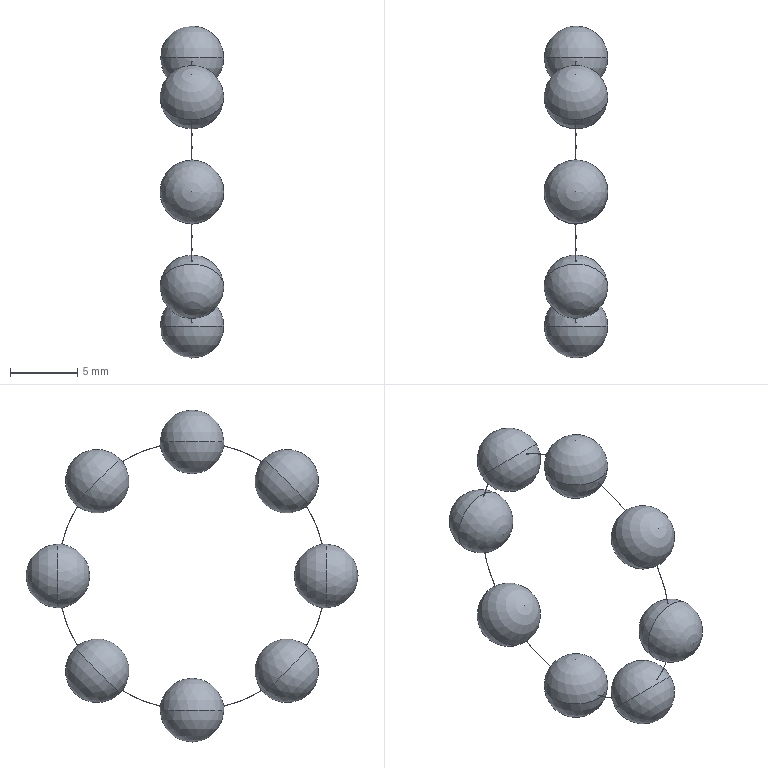Part | SolidWorks | features BaseBody 1 | 1 solid | 32 faces | box 4.762 x 24.762 x 24.762 mm | volume 452.339 mm3 | torus 16 | sphere 16
STEP:
#1=CARTESIAN_POINT('',(4.,9.727,2.365));
#2=VERTEX_POINT('',#1);
#3=CARTESIAN_POINT('',(4.,8.55,5.205));
#4=VERTEX_POINT('',#3);
#5=CARTESIAN_POINT('',(4.,0.,0.));
#6=DIRECTION('',(1.,0.,0.));
#7=DIRECTION('',(0.,0.,-1.));
#8=AXIS2_PLACEMENT_3D('',#5,#6,#7);
#9=CIRCLE('',#8,10.01);
#10=EDGE_CURVE('',#2,#4,#9,.T.);
#11=ORIENTED_EDGE('',*,*,#10,.T.);
#12=CARTESIAN_POINT('',(4.,8.534,5.193));
#13=VERTEX_POINT('',#12);
#14=CARTESIAN_POINT('',(4.,8.55,5.205));
#15=CARTESIAN_POINT('',(4.005,8.55,5.205));
#16=CARTESIAN_POINT('',(4.01,8.547,5.202));
#17=CARTESIAN_POINT('',(4.01,8.538,5.196));
#18=CARTESIAN_POINT('',(4.005,8.534,5.193));
#19=CARTESIAN_POINT('',(4.,8.534,5.193));
#20=B_SPLINE_CURVE_WITH_KNOTS('',3,(#14,#15,#16,#17,#18,#19),.UNSPECIFIED.,.F.,.F.,(4,2,4),(0.,0.5,1.),.UNSPECIFIED.);
#21=EDGE_CURVE('',#4,#13,#20,.T.);
#22=ORIENTED_EDGE('',*,*,#21,.T.);
#23=CARTESIAN_POINT('',(4.,9.707,2.363));
#24=VERTEX_POINT('',#23);
#25=CARTESIAN_POINT('',(4.,0.,0.));
#26=DIRECTION('',(-1.,0.,0.));
#27=DIRECTION('',(0.,0.,-1.));
#28=AXIS2_PLACEMENT_3D('',#25,#26,#27);
#29=CIRCLE('',#28,9.99);
#30=EDGE_CURVE('',#13,#24,#29,.T.);
#31=ORIENTED_EDGE('',*,*,#30,.T.);
#32=CARTESIAN_POINT('',(4.,9.707,2.363));
#33=CARTESIAN_POINT('',(4.005,9.707,2.362));
#34=CARTESIAN_POINT('',(4.01,9.711,2.363));
#35=CARTESIAN_POINT('',(4.01,9.722,2.365));
#36=CARTESIAN_POINT('',(4.005,9.726,2.366));
#37=CARTESIAN_POINT('',(4.,9.727,2.365));
#38=B_SPLINE_CURVE_WITH_KNOTS('',3,(#32,#33,#34,#35,#36,#37),.UNSPECIFIED.,.F.,.F.,(4,2,4),(0.,0.5,1.),.UNSPECIFIED.);
#39=EDGE_CURVE('',#24,#2,#38,.T.);
#40=ORIENTED_EDGE('',*,*,#39,.T.);
#41=EDGE_LOOP('',(#11,#22,#31,#40));
#42=FACE_OUTER_BOUND('',#41,.T.);
#43=CARTESIAN_POINT('',(4.,0.,0.));
#44=DIRECTION('',(1.,0.,0.));
#45=DIRECTION('',(0.,0.,-1.));
#46=AXIS2_PLACEMENT_3D('',#43,#44,#45);
#47=TOROIDAL_SURFACE('',#46,10.,0.01);
#48=ADVANCED_FACE('',(#42),#47,.T.);
#49=CARTESIAN_POINT('',(4.,-2.365,9.727));
#50=VERTEX_POINT('',#49);
#51=CARTESIAN_POINT('',(4.,-5.205,8.55));
#52=VERTEX_POINT('',#51);
#53=CARTESIAN_POINT('',(4.,0.,0.));
#54=DIRECTION('',(1.,0.,0.));
#55=DIRECTION('',(0.,0.,-1.));
#56=AXIS2_PLACEMENT_3D('',#53,#54,#55);
#57=CIRCLE('',#56,10.01);
#58=EDGE_CURVE('',#50,#52,#57,.T.);
#59=ORIENTED_EDGE('',*,*,#58,.T.);
#60=CARTESIAN_POINT('',(4.,-5.193,8.534));
#61=VERTEX_POINT('',#60);
#62=CARTESIAN_POINT('',(4.,-5.205,8.55));
#63=CARTESIAN_POINT('',(4.005,-5.205,8.55));
#64=CARTESIAN_POINT('',(4.01,-5.202,8.547));
#65=CARTESIAN_POINT('',(4.01,-5.196,8.538));
#66=CARTESIAN_POINT('',(4.005,-5.193,8.534));
#67=CARTESIAN_POINT('',(4.,-5.193,8.534));
#68=B_SPLINE_CURVE_WITH_KNOTS('',3,(#62,#63,#64,#65,#66,#67),.UNSPECIFIED.,.F.,.F.,(4,2,4),(0.,0.5,1.),.UNSPECIFIED.);
#69=EDGE_CURVE('',#52,#61,#68,.T.);
#70=ORIENTED_EDGE('',*,*,#69,.T.);
#71=CARTESIAN_POINT('',(4.,-2.363,9.707));
#72=VERTEX_POINT('',#71);
#73=CARTESIAN_POINT('',(4.,0.,0.));
#74=DIRECTION('',(-1.,0.,0.));
#75=DIRECTION('',(0.,0.,-1.));
#76=AXIS2_PLACEMENT_3D('',#73,#74,#75);
#77=CIRCLE('',#76,9.99);
#78=EDGE_CURVE('',#61,#72,#77,.T.);
#79=ORIENTED_EDGE('',*,*,#78,.T.);
#80=CARTESIAN_POINT('',(4.,-2.363,9.707));
#81=CARTESIAN_POINT('',(4.005,-2.362,9.707));
#82=CARTESIAN_POINT('',(4.01,-2.363,9.711));
#83=CARTESIAN_POINT('',(4.01,-2.365,9.722));
#84=CARTESIAN_POINT('',(4.005,-2.366,9.726));
#85=CARTESIAN_POINT('',(4.,-2.365,9.727));
#86=B_SPLINE_CURVE_WITH_KNOTS('',3,(#80,#81,#82,#83,#84,#85),.UNSPECIFIED.,.F.,.F.,(4,2,4),(0.,0.5,1.),.UNSPECIFIED.);
#87=EDGE_CURVE('',#72,#50,#86,.T.);
#88=ORIENTED_EDGE('',*,*,#87,.T.);
#89=EDGE_LOOP('',(#59,#70,#79,#88));
#90=FACE_OUTER_BOUND('',#89,.T.);
#91=CARTESIAN_POINT('',(4.,0.,0.));
#92=DIRECTION('',(1.,0.,0.));
#93=DIRECTION('',(0.,0.,-1.));
#94=AXIS2_PLACEMENT_3D('',#91,#92,#93);
#95=TOROIDAL_SURFACE('',#94,10.,0.01);
#96=ADVANCED_FACE('',(#90),#95,.T.);
#97=CARTESIAN_POINT('',(4.,-8.55,5.205));
#98=VERTEX_POINT('',#97);
#99=CARTESIAN_POINT('',(4.,-9.727,2.365));
#100=VERTEX_POINT('',#99);
#101=CARTESIAN_POINT('',(4.,0.,0.));
#102=DIRECTION('',(1.,0.,0.));
#103=DIRECTION('',(0.,0.,-1.));
#104=AXIS2_PLACEMENT_3D('',#101,#102,#103);
#105=CIRCLE('',#104,10.01);
#106=EDGE_CURVE('',#98,#100,#105,.T.);
#107=ORIENTED_EDGE('',*,*,#106,.T.);
#108=CARTESIAN_POINT('',(4.,-9.707,2.363));
#109=VERTEX_POINT('',#108);
#110=CARTESIAN_POINT('',(4.,-9.727,2.365));
#111=CARTESIAN_POINT('',(4.005,-9.726,2.366));
#112=CARTESIAN_POINT('',(4.01,-9.722,2.365));
#113=CARTESIAN_POINT('',(4.01,-9.711,2.363));
#114=CARTESIAN_POINT('',(4.005,-9.707,2.362));
#115=CARTESIAN_POINT('',(4.,-9.707,2.363));
#116=B_SPLINE_CURVE_WITH_KNOTS('',3,(#110,#111,#112,#113,#114,#115),.UNSPECIFIED.,.F.,.F.,(4,2,4),(0.,0.5,1.),.UNSPECIFIED.);
#117=EDGE_CURVE('',#100,#109,#116,.T.);
#118=ORIENTED_EDGE('',*,*,#117,.T.);
#119=CARTESIAN_POINT('',(4.,-8.534,5.193));
#120=VERTEX_POINT('',#119);
#121=CARTESIAN_POINT('',(4.,0.,0.));
#122=DIRECTION('',(-1.,0.,0.));
#123=DIRECTION('',(0.,0.,-1.));
#124=AXIS2_PLACEMENT_3D('',#121,#122,#123);
#125=CIRCLE('',#124,9.99);
#126=EDGE_CURVE('',#109,#120,#125,.T.);
#127=ORIENTED_EDGE('',*,*,#126,.T.);
#128=CARTESIAN_POINT('',(4.,-8.534,5.193));
#129=CARTESIAN_POINT('',(4.005,-8.534,5.193));
#130=CARTESIAN_POINT('',(4.01,-8.538,5.196));
#131=CARTESIAN_POINT('',(4.01,-8.547,5.202));
#132=CARTESIAN_POINT('',(4.005,-8.55,5.205));
#133=CARTESIAN_POINT('',(4.,-8.55,5.205));
#134=B_SPLINE_CURVE_WITH_KNOTS('',3,(#128,#129,#130,#131,#132,#133),.UNSPECIFIED.,.F.,.F.,(4,2,4),(0.,0.5,1.),.UNSPECIFIED.);
#135=EDGE_CURVE('',#120,#98,#134,.T.);
#136=ORIENTED_EDGE('',*,*,#135,.T.);
#137=EDGE_LOOP('',(#107,#118,#127,#136));
#138=FACE_OUTER_BOUND('',#137,.T.);
#139=CARTESIAN_POINT('',(4.,0.,0.));
#140=DIRECTION('',(1.,0.,0.));
#141=DIRECTION('',(0.,0.,-1.));
#142=AXIS2_PLACEMENT_3D('',#139,#140,#141);
#143=TOROIDAL_SURFACE('',#142,10.,0.01);
#144=ADVANCED_FACE('',(#138),#143,.T.);
#145=CARTESIAN_POINT('',(4.,-9.727,-2.365));
#146=VERTEX_POINT('',#145);
#147=CARTESIAN_POINT('',(4.,-8.55,-5.205));
#148=VERTEX_POINT('',#147);
#149=CARTESIAN_POINT('',(4.,0.,0.));
#150=DIRECTION('',(1.,0.,0.));
#151=DIRECTION('',(0.,0.,-1.));
#152=AXIS2_PLACEMENT_3D('',#149,#150,#151);
#153=CIRCLE('',#152,10.01);
#154=EDGE_CURVE('',#146,#148,#153,.T.);
#155=ORIENTED_EDGE('',*,*,#154,.T.);
#156=CARTESIAN_POINT('',(4.,-8.534,-5.193));
#157=VERTEX_POINT('',#156);
#158=CARTESIAN_POINT('',(4.,-8.55,-5.205));
#159=CARTESIAN_POINT('',(4.005,-8.55,-5.205));
#160=CARTESIAN_POINT('',(4.01,-8.547,-5.202));
#161=CARTESIAN_POINT('',(4.01,-8.538,-5.196));
#162=CARTESIAN_POINT('',(4.005,-8.534,-5.193));
#163=CARTESIAN_POINT('',(4.,-8.534,-5.193));
#164=B_SPLINE_CURVE_WITH_KNOTS('',3,(#158,#159,#160,#161,#162,#163),.UNSPECIFIED.,.F.,.F.,(4,2,4),(0.,0.5,1.),.UNSPECIFIED.);
#165=EDGE_CURVE('',#148,#157,#164,.T.);
#166=ORIENTED_EDGE('',*,*,#165,.T.);
#167=CARTESIAN_POINT('',(4.,-9.707,-2.363));
#168=VERTEX_POINT('',#167);
#169=CARTESIAN_POINT('',(4.,0.,0.));
#170=DIRECTION('',(-1.,0.,0.));
#171=DIRECTION('',(0.,0.,-1.));
#172=AXIS2_PLACEMENT_3D('',#169,#170,#171);
#173=CIRCLE('',#172,9.99);
#174=EDGE_CURVE('',#157,#168,#173,.T.);
#175=ORIENTED_EDGE('',*,*,#174,.T.);
#176=CARTESIAN_POINT('',(4.,-9.707,-2.363));
#177=CARTESIAN_POINT('',(4.005,-9.707,-2.362));
#178=CARTESIAN_POINT('',(4.01,-9.711,-2.363));
#179=CARTESIAN_POINT('',(4.01,-9.722,-2.365));
#180=CARTESIAN_POINT('',(4.005,-9.726,-2.366));
#181=CARTESIAN_POINT('',(4.,-9.727,-2.365));
#182=B_SPLINE_CURVE_WITH_KNOTS('',3,(#176,#177,#178,#179,#180,#181),.UNSPECIFIED.,.F.,.F.,(4,2,4),(0.,0.5,1.),.UNSPECIFIED.);
#183=EDGE_CURVE('',#168,#146,#182,.T.);
#184=ORIENTED_EDGE('',*,*,#183,.T.);
#185=EDGE_LOOP('',(#155,#166,#175,#184));
#186=FACE_OUTER_BOUND('',#185,.T.);
#187=CARTESIAN_POINT('',(4.,0.,0.));
#188=DIRECTION('',(1.,0.,0.));
#189=DIRECTION('',(0.,0.,-1.));
#190=AXIS2_PLACEMENT_3D('',#187,#188,#189);
#191=TOROIDAL_SURFACE('',#190,10.,0.01);
#192=ADVANCED_FACE('',(#186),#191,.T.);
#193=CARTESIAN_POINT('',(4.,-5.205,-8.55));
#194=VERTEX_POINT('',#193);
#195=CARTESIAN_POINT('',(4.,-2.365,-9.727));
#196=VERTEX_POINT('',#195);
#197=CARTESIAN_POINT('',(4.,0.,0.));
#198=DIRECTION('',(1.,0.,0.));
#199=DIRECTION('',(0.,0.,-1.));
#200=AXIS2_PLACEMENT_3D('',#197,#198,#199);
#201=CIRCLE('',#200,10.01);
#202=EDGE_CURVE('',#194,#196,#201,.T.);
#203=ORIENTED_EDGE('',*,*,#202,.T.);
#204=CARTESIAN_POINT('',(4.,-2.363,-9.707));
#205=VERTEX_POINT('',#204);
#206=CARTESIAN_POINT('',(4.,-2.365,-9.727));
#207=CARTESIAN_POINT('',(4.005,-2.366,-9.726));
#208=CARTESIAN_POINT('',(4.01,-2.365,-9.722));
#209=CARTESIAN_POINT('',(4.01,-2.363,-9.711));
#210=CARTESIAN_POINT('',(4.005,-2.362,-9.707));
#211=CARTESIAN_POINT('',(4.,-2.363,-9.707));
#212=B_SPLINE_CURVE_WITH_KNOTS('',3,(#206,#207,#208,#209,#210,#211),.UNSPECIFIED.,.F.,.F.,(4,2,4),(0.,0.5,1.),.UNSPECIFIED.);
#213=EDGE_CURVE('',#196,#205,#212,.T.);
#214=ORIENTED_EDGE('',*,*,#213,.T.);
#215=CARTESIAN_POINT('',(4.,-5.193,-8.534));
#216=VERTEX_POINT('',#215);
#217=CARTESIAN_POINT('',(4.,0.,0.));
#218=DIRECTION('',(-1.,0.,0.));
#219=DIRECTION('',(0.,0.,-1.));
#220=AXIS2_PLACEMENT_3D('',#217,#218,#219);
#221=CIRCLE('',#220,9.99);
#222=EDGE_CURVE('',#205,#216,#221,.T.);
#223=ORIENTED_EDGE('',*,*,#222,.T.);
#224=CARTESIAN_POINT('',(4.,-5.193,-8.534));
#225=CARTESIAN_POINT('',(4.005,-5.193,-8.534));
#226=CARTESIAN_POINT('',(4.01,-5.196,-8.538));
#227=CARTESIAN_POINT('',(4.01,-5.202,-8.547));
#228=CARTESIAN_POINT('',(4.005,-5.205,-8.55));
#229=CARTESIAN_POINT('',(4.,-5.205,-8.55));
#230=B_SPLINE_CURVE_WITH_KNOTS('',3,(#224,#225,#226,#227,#228,#229),.UNSPECIFIED.,.F.,.F.,(4,2,4),(0.,0.5,1.),.UNSPECIFIED.);
#231=EDGE_CURVE('',#216,#194,#230,.T.);
#232=ORIENTED_EDGE('',*,*,#231,.T.);
#233=EDGE_LOOP('',(#203,#214,#223,#232));
#234=FACE_OUTER_BOUND('',#233,.T.);
#235=CARTESIAN_POINT('',(4.,0.,0.));
#236=DIRECTION('',(1.,0.,0.));
#237=DIRECTION('',(0.,0.,-1.));
#238=AXIS2_PLACEMENT_3D('',#235,#236,#237);
#239=TOROIDAL_SURFACE('',#238,10.,0.01);
#240=ADVANCED_FACE('',(#234),#239,.T.);
#241=CARTESIAN_POINT('',(4.,2.365,-9.727));
#242=VERTEX_POINT('',#241);
#243=CARTESIAN_POINT('',(4.,5.205,-8.55));
#244=VERTEX_POINT('',#243);
#245=CARTESIAN_POINT('',(4.,0.,0.));
#246=DIRECTION('',(1.,0.,0.));
#247=DIRECTION('',(0.,0.,-1.));
#248=AXIS2_PLACEMENT_3D('',#245,#246,#247);
#249=CIRCLE('',#248,10.01);
#250=EDGE_CURVE('',#242,#244,#249,.T.);
#251=ORIENTED_EDGE('',*,*,#250,.T.);
#252=CARTESIAN_POINT('',(4.,5.193,-8.534));
#253=VERTEX_POINT('',#252);
#254=CARTESIAN_POINT('',(4.,5.205,-8.55));
#255=CARTESIAN_POINT('',(4.005,5.205,-8.55));
#256=CARTESIAN_POINT('',(4.01,5.202,-8.547));
#257=CARTESIAN_POINT('',(4.01,5.196,-8.538));
#258=CARTESIAN_POINT('',(4.005,5.193,-8.534));
#259=CARTESIAN_POINT('',(4.,5.193,-8.534));
#260=B_SPLINE_CURVE_WITH_KNOTS('',3,(#254,#255,#256,#257,#258,#259),.UNSPECIFIED.,.F.,.F.,(4,2,4),(0.,0.5,1.),.UNSPECIFIED.);
#261=EDGE_CURVE('',#244,#253,#260,.T.);
#262=ORIENTED_EDGE('',*,*,#261,.T.);
#263=CARTESIAN_POINT('',(4.,2.363,-9.707));
#264=VERTEX_POINT('',#263);
#265=CARTESIAN_POINT('',(4.,0.,0.));
#266=DIRECTION('',(-1.,0.,0.));
#267=DIRECTION('',(0.,0.,-1.));
#268=AXIS2_PLACEMENT_3D('',#265,#266,#267);
#269=CIRCLE('',#268,9.99);
#270=EDGE_CURVE('',#253,#264,#269,.T.);
#271=ORIENTED_EDGE('',*,*,#270,.T.);
#272=CARTESIAN_POINT('',(4.,2.363,-9.707));
#273=CARTESIAN_POINT('',(4.005,2.362,-9.707));
#274=CARTESIAN_POINT('',(4.01,2.363,-9.711));
#275=CARTESIAN_POINT('',(4.01,2.365,-9.722));
#276=CARTESIAN_POINT('',(4.005,2.366,-9.726));
#277=CARTESIAN_POINT('',(4.,2.365,-9.727));
#278=B_SPLINE_CURVE_WITH_KNOTS('',3,(#272,#273,#274,#275,#276,#277),.UNSPECIFIED.,.F.,.F.,(4,2,4),(0.,0.5,1.),.UNSPECIFIED.);
#279=EDGE_CURVE('',#264,#242,#278,.T.);
#280=ORIENTED_EDGE('',*,*,#279,.T.);
#281=EDGE_LOOP('',(#251,#262,#271,#280));
#282=FACE_OUTER_BOUND('',#281,.T.);
#283=CARTESIAN_POINT('',(4.,0.,0.));
#284=DIRECTION('',(1.,0.,0.));
#285=DIRECTION('',(0.,0.,-1.));
#286=AXIS2_PLACEMENT_3D('',#283,#284,#285);
#287=TOROIDAL_SURFACE('',#286,10.,0.01);
#288=ADVANCED_FACE('',(#282),#287,.T.);
#289=CARTESIAN_POINT('',(4.,8.55,-5.205));
#290=VERTEX_POINT('',#289);
#291=CARTESIAN_POINT('',(4.,9.727,-2.365));
#292=VERTEX_POINT('',#291);
#293=CARTESIAN_POINT('',(4.,0.,0.));
#294=DIRECTION('',(1.,0.,0.));
#295=DIRECTION('',(0.,0.,-1.));
#296=AXIS2_PLACEMENT_3D('',#293,#294,#295);
#297=CIRCLE('',#296,10.01);
#298=EDGE_CURVE('',#290,#292,#297,.T.);
#299=ORIENTED_EDGE('',*,*,#298,.T.);
#300=CARTESIAN_POINT('',(4.,9.707,-2.363));
#301=VERTEX_POINT('',#300);
#302=CARTESIAN_POINT('',(4.,9.727,-2.365));
#303=CARTESIAN_POINT('',(4.005,9.726,-2.366));
#304=CARTESIAN_POINT('',(4.01,9.722,-2.365));
#305=CARTESIAN_POINT('',(4.01,9.711,-2.363));
#306=CARTESIAN_POINT('',(4.005,9.707,-2.362));
#307=CARTESIAN_POINT('',(4.,9.707,-2.363));
#308=B_SPLINE_CURVE_WITH_KNOTS('',3,(#302,#303,#304,#305,#306,#307),.UNSPECIFIED.,.F.,.F.,(4,2,4),(0.,0.5,1.),.UNSPECIFIED.);
#309=EDGE_CURVE('',#292,#301,#308,.T.);
#310=ORIENTED_EDGE('',*,*,#309,.T.);
#311=CARTESIAN_POINT('',(4.,8.534,-5.193));
#312=VERTEX_POINT('',#311);
#313=CARTESIAN_POINT('',(4.,0.,0.));
#314=DIRECTION('',(-1.,0.,0.));
#315=DIRECTION('',(0.,0.,-1.));
#316=AXIS2_PLACEMENT_3D('',#313,#314,#315);
#317=CIRCLE('',#316,9.99);
#318=EDGE_CURVE('',#301,#312,#317,.T.);
#319=ORIENTED_EDGE('',*,*,#318,.T.);
#320=CARTESIAN_POINT('',(4.,8.534,-5.193));
#321=CARTESIAN_POINT('',(4.005,8.534,-5.193));
#322=CARTESIAN_POINT('',(4.01,8.538,-5.196));
#323=CARTESIAN_POINT('',(4.01,8.547,-5.202));
#324=CARTESIAN_POINT('',(4.005,8.55,-5.205));
#325=CARTESIAN_POINT('',(4.,8.55,-5.205));
#326=B_SPLINE_CURVE_WITH_KNOTS('',3,(#320,#321,#322,#323,#324,#325),.UNSPECIFIED.,.F.,.F.,(4,2,4),(0.,0.5,1.),.UNSPECIFIED.);
#327=EDGE_CURVE('',#312,#290,#326,.T.);
#328=ORIENTED_EDGE('',*,*,#327,.T.);
#329=EDGE_LOOP('',(#299,#310,#319,#328));
#330=FACE_OUTER_BOUND('',#329,.T.);
#331=CARTESIAN_POINT('',(4.,0.,0.));
#332=DIRECTION('',(1.,0.,0.));
#333=DIRECTION('',(0.,0.,-1.));
#334=AXIS2_PLACEMENT_3D('',#331,#332,#333);
#335=TOROIDAL_SURFACE('',#334,10.,0.01);
#336=ADVANCED_FACE('',(#330),#335,.T.);
#337=CARTESIAN_POINT('',(4.,5.205,8.55));
#338=VERTEX_POINT('',#337);
#339=CARTESIAN_POINT('',(4.,2.365,9.727));
#340=VERTEX_POINT('',#339);
#341=CARTESIAN_POINT('',(4.,0.,0.));
#342=DIRECTION('',(1.,0.,0.));
#343=DIRECTION('',(0.,0.,-1.));
#344=AXIS2_PLACEMENT_3D('',#341,#342,#343);
#345=CIRCLE('',#344,10.01);
#346=EDGE_CURVE('',#338,#340,#345,.T.);
#347=ORIENTED_EDGE('',*,*,#346,.T.);
#348=CARTESIAN_POINT('',(4.,2.363,9.707));
#349=VERTEX_POINT('',#348);
#350=CARTESIAN_POINT('',(4.,2.365,9.727));
#351=CARTESIAN_POINT('',(4.005,2.366,9.726));
#352=CARTESIAN_POINT('',(4.01,2.365,9.722));
#353=CARTESIAN_POINT('',(4.01,2.363,9.711));
#354=CARTESIAN_POINT('',(4.005,2.362,9.707));
#355=CARTESIAN_POINT('',(4.,2.363,9.707));
#356=B_SPLINE_CURVE_WITH_KNOTS('',3,(#350,#351,#352,#353,#354,#355),.UNSPECIFIED.,.F.,.F.,(4,2,4),(0.,0.5,1.),.UNSPECIFIED.);
#357=EDGE_CURVE('',#340,#349,#356,.T.);
#358=ORIENTED_EDGE('',*,*,#357,.T.);
#359=CARTESIAN_POINT('',(4.,5.193,8.534));
#360=VERTEX_POINT('',#359);
#361=CARTESIAN_POINT('',(4.,0.,0.));
#362=DIRECTION('',(-1.,0.,0.));
#363=DIRECTION('',(0.,0.,-1.));
#364=AXIS2_PLACEMENT_3D('',#361,#362,#363);
#365=CIRCLE('',#364,9.99);
#366=EDGE_CURVE('',#349,#360,#365,.T.);
#367=ORIENTED_EDGE('',*,*,#366,.T.);
#368=CARTESIAN_POINT('',(4.,5.193,8.534));
#369=CARTESIAN_POINT('',(4.005,5.193,8.534));
#370=CARTESIAN_POINT('',(4.01,5.196,8.538));
#371=CARTESIAN_POINT('',(4.01,5.202,8.547));
#372=CARTESIAN_POINT('',(4.005,5.205,8.55));
#373=CARTESIAN_POINT('',(4.,5.205,8.55));
#374=B_SPLINE_CURVE_WITH_KNOTS('',3,(#368,#369,#370,#371,#372,#373),.UNSPECIFIED.,.F.,.F.,(4,2,4),(0.,0.5,1.),.UNSPECIFIED.);
#375=EDGE_CURVE('',#360,#338,#374,.T.);
#376=ORIENTED_EDGE('',*,*,#375,.T.);
#377=EDGE_LOOP('',(#347,#358,#367,#376));
#378=FACE_OUTER_BOUND('',#377,.T.);
#379=CARTESIAN_POINT('',(4.,0.,0.));
#380=DIRECTION('',(1.,0.,0.));
#381=DIRECTION('',(0.,0.,-1.));
#382=AXIS2_PLACEMENT_3D('',#379,#380,#381);
#383=TOROIDAL_SURFACE('',#382,10.,0.01);
#384=ADVANCED_FACE('',(#378),#383,.T.);
#385=CARTESIAN_POINT('',(4.,9.727,2.365));
#386=CARTESIAN_POINT('',(3.995,9.726,2.366));
#387=CARTESIAN_POINT('',(3.99,9.722,2.365));
#388=CARTESIAN_POINT('',(3.99,9.711,2.363));
#389=CARTESIAN_POINT('',(3.995,9.707,2.362));
#390=CARTESIAN_POINT('',(4.,9.707,2.363));
#391=B_SPLINE_CURVE_WITH_KNOTS('',3,(#385,#386,#387,#388,#389,#390),.UNSPECIFIED.,.F.,.F.,(4,2,4),(0.,0.5,1.),.UNSPECIFIED.);
#392=EDGE_CURVE('',#2,#24,#391,.T.);
#393=ORIENTED_EDGE('',*,*,#392,.F.);
#394=ORIENTED_EDGE('',*,*,#39,.F.);
#395=EDGE_LOOP('',(#393,#394));
#396=FACE_BOUND('',#395,.T.);
#397=ORIENTED_EDGE('',*,*,#309,.F.);
#398=CARTESIAN_POINT('',(4.,9.707,-2.363));
#399=CARTESIAN_POINT('',(3.995,9.707,-2.362));
#400=CARTESIAN_POINT('',(3.99,9.711,-2.363));
#401=CARTESIAN_POINT('',(3.99,9.722,-2.365));
#402=CARTESIAN_POINT('',(3.995,9.726,-2.366));
#403=CARTESIAN_POINT('',(4.,9.727,-2.365));
#404=B_SPLINE_CURVE_WITH_KNOTS('',3,(#398,#399,#400,#401,#402,#403),.UNSPECIFIED.,.F.,.F.,(4,2,4),(0.,0.5,1.),.UNSPECIFIED.);
#405=EDGE_CURVE('',#301,#292,#404,.T.);
#406=ORIENTED_EDGE('',*,*,#405,.F.);
#407=EDGE_LOOP('',(#397,#406));
#408=FACE_BOUND('',#407,.T.);
#409=CARTESIAN_POINT('',(4.,10.,2.381));
#410=VERTEX_POINT('',#409);
#411=CARTESIAN_POINT('',(4.,10.,-2.381));
#412=VERTEX_POINT('',#411);
#413=CARTESIAN_POINT('',(4.,10.,0.));
#414=DIRECTION('',(0.,-1.,0.));
#415=DIRECTION('',(0.,0.,1.));
#416=AXIS2_PLACEMENT_3D('',#413,#414,#415);
#417=CIRCLE('',#416,2.381);
#418=EDGE_CURVE('',#410,#412,#417,.T.);
#419=ORIENTED_EDGE('',*,*,#418,.T.);
#420=CARTESIAN_POINT('',(4.,10.,0.));
#421=DIRECTION('',(0.,-1.,0.));
#422=DIRECTION('',(0.,0.,1.));
#423=AXIS2_PLACEMENT_3D('',#420,#421,#422);
#424=CIRCLE('',#423,2.381);
#425=EDGE_CURVE('',#412,#410,#424,.T.);
#426=ORIENTED_EDGE('',*,*,#425,.T.);
#427=EDGE_LOOP('',(#419,#426));
#428=FACE_OUTER_BOUND('',#427,.T.);
#429=CARTESIAN_POINT('',(4.,10.,0.));
#430=DIRECTION('',(0.,1.,0.));
#431=DIRECTION('',(1.,0.,0.));
#432=AXIS2_PLACEMENT_3D('',#429,#430,#431);
#433=SPHERICAL_SURFACE('',#432,2.381);
#434=ADVANCED_FACE('',(#396,#408,#428),#433,.T.);
#435=CARTESIAN_POINT('',(4.,5.205,8.55));
#436=CARTESIAN_POINT('',(3.995,5.205,8.55));
#437=CARTESIAN_POINT('',(3.99,5.202,8.547));
#438=CARTESIAN_POINT('',(3.99,5.196,8.538));
#439=CARTESIAN_POINT('',(3.995,5.193,8.534));
#440=CARTESIAN_POINT('',(4.,5.193,8.534));
#441=B_SPLINE_CURVE_WITH_KNOTS('',3,(#435,#436,#437,#438,#439,#440),.UNSPECIFIED.,.F.,.F.,(4,2,4),(0.,0.5,1.),.UNSPECIFIED.);
#442=EDGE_CURVE('',#338,#360,#441,.T.);
#443=ORIENTED_EDGE('',*,*,#442,.F.);
#444=ORIENTED_EDGE('',*,*,#375,.F.);
#445=EDGE_LOOP('',(#443,#444));
#446=FACE_BOUND('',#445,.T.);
#447=ORIENTED_EDGE('',*,*,#21,.F.);
#448=CARTESIAN_POINT('',(4.,8.534,5.193));
#449=CARTESIAN_POINT('',(3.995,8.534,5.193));
#450=CARTESIAN_POINT('',(3.99,8.538,5.196));
#451=CARTESIAN_POINT('',(3.99,8.547,5.202));
#452=CARTESIAN_POINT('',(3.995,8.55,5.205));
#453=CARTESIAN_POINT('',(4.,8.55,5.205));
#454=B_SPLINE_CURVE_WITH_KNOTS('',3,(#448,#449,#450,#451,#452,#453),.UNSPECIFIED.,.F.,.F.,(4,2,4),(0.,0.5,1.),.UNSPECIFIED.);
#455=EDGE_CURVE('',#13,#4,#454,.T.);
#456=ORIENTED_EDGE('',*,*,#455,.F.);
#457=EDGE_LOOP('',(#447,#456));
#458=FACE_BOUND('',#457,.T.);
#459=CARTESIAN_POINT('',(4.,5.387,8.755));
#460=VERTEX_POINT('',#459);
#461=CARTESIAN_POINT('',(4.,8.755,5.387));
#462=VERTEX_POINT('',#461);
#463=CARTESIAN_POINT('',(4.,7.071,7.071));
#464=DIRECTION('',(0.,-0.7071,-0.7071));
#465=DIRECTION('',(0.,-0.7071,0.7071));
#466=AXIS2_PLACEMENT_3D('',#463,#464,#465);
#467=CIRCLE('',#466,2.381);
#468=EDGE_CURVE('',#460,#462,#467,.T.);
#469=ORIENTED_EDGE('',*,*,#468,.T.);
#470=CARTESIAN_POINT('',(4.,7.071,7.071));
#471=DIRECTION('',(0.,-0.7071,-0.7071));
#472=DIRECTION('',(0.,-0.7071,0.7071));
#473=AXIS2_PLACEMENT_3D('',#470,#471,#472);
#474=CIRCLE('',#473,2.381);
#475=EDGE_CURVE('',#462,#460,#474,.T.);
#476=ORIENTED_EDGE('',*,*,#475,.T.);
#477=EDGE_LOOP('',(#469,#476));
#478=FACE_OUTER_BOUND('',#477,.T.);
#479=CARTESIAN_POINT('',(4.,7.071,7.071));
#480=DIRECTION('',(0.,0.7071,0.7071));
#481=DIRECTION('',(1.,0.,0.));
#482=AXIS2_PLACEMENT_3D('',#479,#480,#481);
#483=SPHERICAL_SURFACE('',#482,2.381);
#484=ADVANCED_FACE('',(#446,#458,#478),#483,.T.);
#485=CARTESIAN_POINT('',(4.,-2.365,9.727));
#486=CARTESIAN_POINT('',(3.995,-2.366,9.726));
#487=CARTESIAN_POINT('',(3.99,-2.365,9.722));
#488=CARTESIAN_POINT('',(3.99,-2.363,9.711));
#489=CARTESIAN_POINT('',(3.995,-2.362,9.707));
#490=CARTESIAN_POINT('',(4.,-2.363,9.707));
#491=B_SPLINE_CURVE_WITH_KNOTS('',3,(#485,#486,#487,#488,#489,#490),.UNSPECIFIED.,.F.,.F.,(4,2,4),(0.,0.5,1.),.UNSPECIFIED.);
#492=EDGE_CURVE('',#50,#72,#491,.T.);
#493=ORIENTED_EDGE('',*,*,#492,.F.);
#494=ORIENTED_EDGE('',*,*,#87,.F.);
#495=EDGE_LOOP('',(#493,#494));
#496=FACE_BOUND('',#495,.T.);
#497=ORIENTED_EDGE('',*,*,#357,.F.);
#498=CARTESIAN_POINT('',(4.,2.363,9.707));
#499=CARTESIAN_POINT('',(3.995,2.362,9.707));
#500=CARTESIAN_POINT('',(3.99,2.363,9.711));
#501=CARTESIAN_POINT('',(3.99,2.365,9.722));
#502=CARTESIAN_POINT('',(3.995,2.366,9.726));
#503=CARTESIAN_POINT('',(4.,2.365,9.727));
#504=B_SPLINE_CURVE_WITH_KNOTS('',3,(#498,#499,#500,#501,#502,#503),.UNSPECIFIED.,.F.,.F.,(4,2,4),(0.,0.5,1.),.UNSPECIFIED.);
#505=EDGE_CURVE('',#349,#340,#504,.T.);
#506=ORIENTED_EDGE('',*,*,#505,.F.);
#507=EDGE_LOOP('',(#497,#506));
#508=FACE_BOUND('',#507,.T.);
#509=CARTESIAN_POINT('',(4.,-2.381,10.));
#510=VERTEX_POINT('',#509);
#511=CARTESIAN_POINT('',(4.,2.381,10.));
#512=VERTEX_POINT('',#511);
#513=CARTESIAN_POINT('',(4.,0.,10.));
#514=DIRECTION('',(0.,0.,-1.));
#515=DIRECTION('',(0.,-1.,0.));
#516=AXIS2_PLACEMENT_3D('',#513,#514,#515);
#517=CIRCLE('',#516,2.381);
#518=EDGE_CURVE('',#510,#512,#517,.T.);
#519=ORIENTED_EDGE('',*,*,#518,.T.);
#520=CARTESIAN_POINT('',(4.,0.,10.));
#521=DIRECTION('',(0.,0.,-1.));
#522=DIRECTION('',(0.,-1.,0.));
#523=AXIS2_PLACEMENT_3D('',#520,#521,#522);
#524=CIRCLE('',#523,2.381);
#525=EDGE_CURVE('',#512,#510,#524,.T.);
#526=ORIENTED_EDGE('',*,*,#525,.T.);
#527=EDGE_LOOP('',(#519,#526));
#528=FACE_OUTER_BOUND('',#527,.T.);
#529=CARTESIAN_POINT('',(4.,0.,10.));
#530=DIRECTION('',(0.,0.,1.));
#531=DIRECTION('',(1.,0.,0.));
#532=AXIS2_PLACEMENT_3D('',#529,#530,#531);
#533=SPHERICAL_SURFACE('',#532,2.381);
#534=ADVANCED_FACE('',(#496,#508,#528),#533,.T.);
#535=CARTESIAN_POINT('',(4.,-8.55,5.205));
#536=CARTESIAN_POINT('',(3.995,-8.55,5.205));
#537=CARTESIAN_POINT('',(3.99,-8.547,5.202));
#538=CARTESIAN_POINT('',(3.99,-8.538,5.196));
#539=CARTESIAN_POINT('',(3.995,-8.534,5.193));
#540=CARTESIAN_POINT('',(4.,-8.534,5.193));
#541=B_SPLINE_CURVE_WITH_KNOTS('',3,(#535,#536,#537,#538,#539,#540),.UNSPECIFIED.,.F.,.F.,(4,2,4),(0.,0.5,1.),.UNSPECIFIED.);
#542=EDGE_CURVE('',#98,#120,#541,.T.);
#543=ORIENTED_EDGE('',*,*,#542,.F.);
#544=ORIENTED_EDGE('',*,*,#135,.F.);
#545=EDGE_LOOP('',(#543,#544));
#546=FACE_BOUND('',#545,.T.);
#547=ORIENTED_EDGE('',*,*,#69,.F.);
#548=CARTESIAN_POINT('',(4.,-5.193,8.534));
#549=CARTESIAN_POINT('',(3.995,-5.193,8.534));
#550=CARTESIAN_POINT('',(3.99,-5.196,8.538));
#551=CARTESIAN_POINT('',(3.99,-5.202,8.547));
#552=CARTESIAN_POINT('',(3.995,-5.205,8.55));
#553=CARTESIAN_POINT('',(4.,-5.205,8.55));
#554=B_SPLINE_CURVE_WITH_KNOTS('',3,(#548,#549,#550,#551,#552,#553),.UNSPECIFIED.,.F.,.F.,(4,2,4),(0.,0.5,1.),.UNSPECIFIED.);
#555=EDGE_CURVE('',#61,#52,#554,.T.);
#556=ORIENTED_EDGE('',*,*,#555,.F.);
#557=EDGE_LOOP('',(#547,#556));
#558=FACE_BOUND('',#557,.T.);
#559=CARTESIAN_POINT('',(4.,-8.755,5.387));
#560=VERTEX_POINT('',#559);
#561=CARTESIAN_POINT('',(4.,-5.387,8.755));
#562=VERTEX_POINT('',#561);
#563=CARTESIAN_POINT('',(4.,-7.071,7.071));
#564=DIRECTION('',(0.,0.7071,-0.7071));
#565=DIRECTION('',(0.,-0.7071,-0.7071));
#566=AXIS2_PLACEMENT_3D('',#563,#564,#565);
#567=CIRCLE('',#566,2.381);
#568=EDGE_CURVE('',#560,#562,#567,.T.);
#569=ORIENTED_EDGE('',*,*,#568,.T.);
#570=CARTESIAN_POINT('',(4.,-7.071,7.071));
#571=DIRECTION('',(0.,0.7071,-0.7071));
#572=DIRECTION('',(0.,-0.7071,-0.7071));
#573=AXIS2_PLACEMENT_3D('',#570,#571,#572);
#574=CIRCLE('',#573,2.381);
#575=EDGE_CURVE('',#562,#560,#574,.T.);
#576=ORIENTED_EDGE('',*,*,#575,.T.);
#577=EDGE_LOOP('',(#569,#576));
#578=FACE_OUTER_BOUND('',#577,.T.);
#579=CARTESIAN_POINT('',(4.,-7.071,7.071));
#580=DIRECTION('',(0.,-0.7071,0.7071));
#581=DIRECTION('',(1.,0.,0.));
#582=AXIS2_PLACEMENT_3D('',#579,#580,#581);
#583=SPHERICAL_SURFACE('',#582,2.381);
#584=ADVANCED_FACE('',(#546,#558,#578),#583,.T.);
#585=CARTESIAN_POINT('',(4.,-9.727,-2.365));
#586=CARTESIAN_POINT('',(3.995,-9.726,-2.366));
#587=CARTESIAN_POINT('',(3.99,-9.722,-2.365));
#588=CARTESIAN_POINT('',(3.99,-9.711,-2.363));
#589=CARTESIAN_POINT('',(3.995,-9.707,-2.362));
#590=CARTESIAN_POINT('',(4.,-9.707,-2.363));
#591=B_SPLINE_CURVE_WITH_KNOTS('',3,(#585,#586,#587,#588,#589,#590),.UNSPECIFIED.,.F.,.F.,(4,2,4),(0.,0.5,1.),.UNSPECIFIED.);
#592=EDGE_CURVE('',#146,#168,#591,.T.);
#593=ORIENTED_EDGE('',*,*,#592,.F.);
#594=ORIENTED_EDGE('',*,*,#183,.F.);
#595=EDGE_LOOP('',(#593,#594));
#596=FACE_BOUND('',#595,.T.);
#597=ORIENTED_EDGE('',*,*,#117,.F.);
#598=CARTESIAN_POINT('',(4.,-9.707,2.363));
#599=CARTESIAN_POINT('',(3.995,-9.707,2.362));
#600=CARTESIAN_POINT('',(3.99,-9.711,2.363));
#601=CARTESIAN_POINT('',(3.99,-9.722,2.365));
#602=CARTESIAN_POINT('',(3.995,-9.726,2.366));
#603=CARTESIAN_POINT('',(4.,-9.727,2.365));
#604=B_SPLINE_CURVE_WITH_KNOTS('',3,(#598,#599,#600,#601,#602,#603),.UNSPECIFIED.,.F.,.F.,(4,2,4),(0.,0.5,1.),.UNSPECIFIED.);
#605=EDGE_CURVE('',#109,#100,#604,.T.);
#606=ORIENTED_EDGE('',*,*,#605,.F.);
#607=EDGE_LOOP('',(#597,#606));
#608=FACE_BOUND('',#607,.T.);
#609=CARTESIAN_POINT('',(4.,-10.,-2.381));
#610=VERTEX_POINT('',#609);
#611=CARTESIAN_POINT('',(4.,-10.,2.381));
#612=VERTEX_POINT('',#611);
#613=CARTESIAN_POINT('',(4.,-10.,0.));
#614=DIRECTION('',(0.,1.,0.));
#615=DIRECTION('',(0.,0.,-1.));
#616=AXIS2_PLACEMENT_3D('',#613,#614,#615);
#617=CIRCLE('',#616,2.381);
#618=EDGE_CURVE('',#610,#612,#617,.T.);
#619=ORIENTED_EDGE('',*,*,#618,.T.);
#620=CARTESIAN_POINT('',(4.,-10.,0.));
#621=DIRECTION('',(0.,1.,0.));
#622=DIRECTION('',(0.,0.,-1.));
#623=AXIS2_PLACEMENT_3D('',#620,#621,#622);
#624=CIRCLE('',#623,2.381);
#625=EDGE_CURVE('',#612,#610,#624,.T.);
#626=ORIENTED_EDGE('',*,*,#625,.T.);
#627=EDGE_LOOP('',(#619,#626));
#628=FACE_OUTER_BOUND('',#627,.T.);
#629=CARTESIAN_POINT('',(4.,-10.,0.));
#630=DIRECTION('',(0.,-1.,0.));
#631=DIRECTION('',(1.,0.,0.));
#632=AXIS2_PLACEMENT_3D('',#629,#630,#631);
#633=SPHERICAL_SURFACE('',#632,2.381);
#634=ADVANCED_FACE('',(#596,#608,#628),#633,.T.);
#635=CARTESIAN_POINT('',(4.,-5.205,-8.55));
#636=CARTESIAN_POINT('',(3.995,-5.205,-8.55));
#637=CARTESIAN_POINT('',(3.99,-5.202,-8.547));
#638=CARTESIAN_POINT('',(3.99,-5.196,-8.538));
#639=CARTESIAN_POINT('',(3.995,-5.193,-8.534));
#640=CARTESIAN_POINT('',(4.,-5.193,-8.534));
#641=B_SPLINE_CURVE_WITH_KNOTS('',3,(#635,#636,#637,#638,#639,#640),.UNSPECIFIED.,.F.,.F.,(4,2,4),(0.,0.5,1.),.UNSPECIFIED.);
#642=EDGE_CURVE('',#194,#216,#641,.T.);
#643=ORIENTED_EDGE('',*,*,#642,.F.);
#644=ORIENTED_EDGE('',*,*,#231,.F.);
#645=EDGE_LOOP('',(#643,#644));
#646=FACE_BOUND('',#645,.T.);
#647=ORIENTED_EDGE('',*,*,#165,.F.);
#648=CARTESIAN_POINT('',(4.,-8.534,-5.193));
#649=CARTESIAN_POINT('',(3.995,-8.534,-5.193));
#650=CARTESIAN_POINT('',(3.99,-8.538,-5.196));
#651=CARTESIAN_POINT('',(3.99,-8.547,-5.202));
#652=CARTESIAN_POINT('',(3.995,-8.55,-5.205));
#653=CARTESIAN_POINT('',(4.,-8.55,-5.205));
#654=B_SPLINE_CURVE_WITH_KNOTS('',3,(#648,#649,#650,#651,#652,#653),.UNSPECIFIED.,.F.,.F.,(4,2,4),(0.,0.5,1.),.UNSPECIFIED.);
#655=EDGE_CURVE('',#157,#148,#654,.T.);
#656=ORIENTED_EDGE('',*,*,#655,.F.);
#657=EDGE_LOOP('',(#647,#656));
#658=FACE_BOUND('',#657,.T.);
#659=CARTESIAN_POINT('',(4.,-5.387,-8.755));
#660=VERTEX_POINT('',#659);
#661=CARTESIAN_POINT('',(4.,-8.755,-5.387));
#662=VERTEX_POINT('',#661);
#663=CARTESIAN_POINT('',(4.,-7.071,-7.071));
#664=DIRECTION('',(0.,0.7071,0.7071));
#665=DIRECTION('',(0.,0.7071,-0.7071));
#666=AXIS2_PLACEMENT_3D('',#663,#664,#665);
#667=CIRCLE('',#666,2.381);
#668=EDGE_CURVE('',#660,#662,#667,.T.);
#669=ORIENTED_EDGE('',*,*,#668,.T.);
#670=CARTESIAN_POINT('',(4.,-7.071,-7.071));
#671=DIRECTION('',(0.,0.7071,0.7071));
#672=DIRECTION('',(0.,0.7071,-0.7071));
#673=AXIS2_PLACEMENT_3D('',#670,#671,#672);
#674=CIRCLE('',#673,2.381);
#675=EDGE_CURVE('',#662,#660,#674,.T.);
#676=ORIENTED_EDGE('',*,*,#675,.T.);
#677=EDGE_LOOP('',(#669,#676));
#678=FACE_OUTER_BOUND('',#677,.T.);
#679=CARTESIAN_POINT('',(4.,-7.071,-7.071));
#680=DIRECTION('',(0.,-0.7071,-0.7071));
#681=DIRECTION('',(1.,0.,0.));
#682=AXIS2_PLACEMENT_3D('',#679,#680,#681);
#683=SPHERICAL_SURFACE('',#682,2.381);
#684=ADVANCED_FACE('',(#646,#658,#678),#683,.T.);
#685=CARTESIAN_POINT('',(4.,2.365,-9.727));
#686=CARTESIAN_POINT('',(3.995,2.366,-9.726));
#687=CARTESIAN_POINT('',(3.99,2.365,-9.722));
#688=CARTESIAN_POINT('',(3.99,2.363,-9.711));
#689=CARTESIAN_POINT('',(3.995,2.362,-9.707));
#690=CARTESIAN_POINT('',(4.,2.363,-9.707));
#691=B_SPLINE_CURVE_WITH_KNOTS('',3,(#685,#686,#687,#688,#689,#690),.UNSPECIFIED.,.F.,.F.,(4,2,4),(0.,0.5,1.),.UNSPECIFIED.);
#692=EDGE_CURVE('',#242,#264,#691,.T.);
#693=ORIENTED_EDGE('',*,*,#692,.F.);
#694=ORIENTED_EDGE('',*,*,#279,.F.);
#695=EDGE_LOOP('',(#693,#694));
#696=FACE_BOUND('',#695,.T.);
#697=ORIENTED_EDGE('',*,*,#213,.F.);
#698=CARTESIAN_POINT('',(4.,-2.363,-9.707));
#699=CARTESIAN_POINT('',(3.995,-2.362,-9.707));
#700=CARTESIAN_POINT('',(3.99,-2.363,-9.711));
#701=CARTESIAN_POINT('',(3.99,-2.365,-9.722));
#702=CARTESIAN_POINT('',(3.995,-2.366,-9.726));
#703=CARTESIAN_POINT('',(4.,-2.365,-9.727));
#704=B_SPLINE_CURVE_WITH_KNOTS('',3,(#698,#699,#700,#701,#702,#703),.UNSPECIFIED.,.F.,.F.,(4,2,4),(0.,0.5,1.),.UNSPECIFIED.);
#705=EDGE_CURVE('',#205,#196,#704,.T.);
#706=ORIENTED_EDGE('',*,*,#705,.F.);
#707=EDGE_LOOP('',(#697,#706));
#708=FACE_BOUND('',#707,.T.);
#709=CARTESIAN_POINT('',(4.,2.381,-10.));
#710=VERTEX_POINT('',#709);
#711=CARTESIAN_POINT('',(4.,-2.381,-10.));
#712=VERTEX_POINT('',#711);
#713=CARTESIAN_POINT('',(4.,0.,-10.));
#714=DIRECTION('',(0.,0.,1.));
#715=DIRECTION('',(0.,1.,0.));
#716=AXIS2_PLACEMENT_3D('',#713,#714,#715);
#717=CIRCLE('',#716,2.381);
#718=EDGE_CURVE('',#710,#712,#717,.T.);
#719=ORIENTED_EDGE('',*,*,#718,.T.);
#720=CARTESIAN_POINT('',(4.,0.,-10.));
#721=DIRECTION('',(0.,0.,1.));
#722=DIRECTION('',(0.,1.,0.));
#723=AXIS2_PLACEMENT_3D('',#720,#721,#722);
#724=CIRCLE('',#723,2.381);
#725=EDGE_CURVE('',#712,#710,#724,.T.);
#726=ORIENTED_EDGE('',*,*,#725,.T.);
#727=EDGE_LOOP('',(#719,#726));
#728=FACE_OUTER_BOUND('',#727,.T.);
#729=CARTESIAN_POINT('',(4.,0.,-10.));
#730=DIRECTION('',(0.,0.,-1.));
#731=DIRECTION('',(1.,0.,0.));
#732=AXIS2_PLACEMENT_3D('',#729,#730,#731);
#733=SPHERICAL_SURFACE('',#732,2.381);
#734=ADVANCED_FACE('',(#696,#708,#728),#733,.T.);
#735=CARTESIAN_POINT('',(4.,8.55,-5.205));
#736=CARTESIAN_POINT('',(3.995,8.55,-5.205));
#737=CARTESIAN_POINT('',(3.99,8.547,-5.202));
#738=CARTESIAN_POINT('',(3.99,8.538,-5.196));
#739=CARTESIAN_POINT('',(3.995,8.534,-5.193));
#740=CARTESIAN_POINT('',(4.,8.534,-5.193));
#741=B_SPLINE_CURVE_WITH_KNOTS('',3,(#735,#736,#737,#738,#739,#740),.UNSPECIFIED.,.F.,.F.,(4,2,4),(0.,0.5,1.),.UNSPECIFIED.);
#742=EDGE_CURVE('',#290,#312,#741,.T.);
#743=ORIENTED_EDGE('',*,*,#742,.F.);
#744=ORIENTED_EDGE('',*,*,#327,.F.);
#745=EDGE_LOOP('',(#743,#744));
#746=FACE_BOUND('',#745,.T.);
#747=ORIENTED_EDGE('',*,*,#261,.F.);
#748=CARTESIAN_POINT('',(4.,5.193,-8.534));
#749=CARTESIAN_POINT('',(3.995,5.193,-8.534));
#750=CARTESIAN_POINT('',(3.99,5.196,-8.538));
#751=CARTESIAN_POINT('',(3.99,5.202,-8.547));
#752=CARTESIAN_POINT('',(3.995,5.205,-8.55));
#753=CARTESIAN_POINT('',(4.,5.205,-8.55));
#754=B_SPLINE_CURVE_WITH_KNOTS('',3,(#748,#749,#750,#751,#752,#753),.UNSPECIFIED.,.F.,.F.,(4,2,4),(0.,0.5,1.),.UNSPECIFIED.);
#755=EDGE_CURVE('',#253,#244,#754,.T.);
#756=ORIENTED_EDGE('',*,*,#755,.F.);
#757=EDGE_LOOP('',(#747,#756));
#758=FACE_BOUND('',#757,.T.);
#759=CARTESIAN_POINT('',(4.,8.755,-5.387));
#760=VERTEX_POINT('',#759);
#761=CARTESIAN_POINT('',(4.,5.387,-8.755));
#762=VERTEX_POINT('',#761);
#763=CARTESIAN_POINT('',(4.,7.071,-7.071));
#764=DIRECTION('',(0.,-0.7071,0.7071));
#765=DIRECTION('',(0.,0.7071,0.7071));
#766=AXIS2_PLACEMENT_3D('',#763,#764,#765);
#767=CIRCLE('',#766,2.381);
#768=EDGE_CURVE('',#760,#762,#767,.T.);
#769=ORIENTED_EDGE('',*,*,#768,.T.);
#770=CARTESIAN_POINT('',(4.,7.071,-7.071));
#771=DIRECTION('',(0.,-0.7071,0.7071));
#772=DIRECTION('',(0.,0.7071,0.7071));
#773=AXIS2_PLACEMENT_3D('',#770,#771,#772);
#774=CIRCLE('',#773,2.381);
#775=EDGE_CURVE('',#762,#760,#774,.T.);
#776=ORIENTED_EDGE('',*,*,#775,.T.);
#777=EDGE_LOOP('',(#769,#776));
#778=FACE_OUTER_BOUND('',#777,.T.);
#779=CARTESIAN_POINT('',(4.,7.071,-7.071));
#780=DIRECTION('',(0.,0.7071,-0.7071));
#781=DIRECTION('',(1.,0.,0.));
#782=AXIS2_PLACEMENT_3D('',#779,#780,#781);
#783=SPHERICAL_SURFACE('',#782,2.381);
#784=ADVANCED_FACE('',(#746,#758,#778),#783,.T.);
#785=ORIENTED_EDGE('',*,*,#768,.F.);
#786=ORIENTED_EDGE('',*,*,#775,.F.);
#787=EDGE_LOOP('',(#785,#786));
#788=FACE_OUTER_BOUND('',#787,.T.);
#789=CARTESIAN_POINT('',(4.,7.071,-7.071));
#790=DIRECTION('',(0.,0.7071,-0.7071));
#791=DIRECTION('',(1.,0.,0.));
#792=AXIS2_PLACEMENT_3D('',#789,#790,#791);
#793=SPHERICAL_SURFACE('',#792,2.381);
#794=ADVANCED_FACE('',(#788),#793,.T.);
#795=ORIENTED_EDGE('',*,*,#718,.F.);
#796=ORIENTED_EDGE('',*,*,#725,.F.);
#797=EDGE_LOOP('',(#795,#796));
#798=FACE_OUTER_BOUND('',#797,.T.);
#799=CARTESIAN_POINT('',(4.,0.,-10.));
#800=DIRECTION('',(0.,0.,-1.));
#801=DIRECTION('',(1.,0.,0.));
#802=AXIS2_PLACEMENT_3D('',#799,#800,#801);
#803=SPHERICAL_SURFACE('',#802,2.381);
#804=ADVANCED_FACE('',(#798),#803,.T.);
#805=ORIENTED_EDGE('',*,*,#668,.F.);
#806=ORIENTED_EDGE('',*,*,#675,.F.);
#807=EDGE_LOOP('',(#805,#806));
#808=FACE_OUTER_BOUND('',#807,.T.);
#809=CARTESIAN_POINT('',(4.,-7.071,-7.071));
#810=DIRECTION('',(0.,-0.7071,-0.7071));
#811=DIRECTION('',(1.,0.,0.));
#812=AXIS2_PLACEMENT_3D('',#809,#810,#811);
#813=SPHERICAL_SURFACE('',#812,2.381);
#814=ADVANCED_FACE('',(#808),#813,.T.);
#815=ORIENTED_EDGE('',*,*,#618,.F.);
#816=ORIENTED_EDGE('',*,*,#625,.F.);
#817=EDGE_LOOP('',(#815,#816));
#818=FACE_OUTER_BOUND('',#817,.T.);
#819=CARTESIAN_POINT('',(4.,-10.,0.));
#820=DIRECTION('',(0.,-1.,0.));
#821=DIRECTION('',(1.,0.,0.));
#822=AXIS2_PLACEMENT_3D('',#819,#820,#821);
#823=SPHERICAL_SURFACE('',#822,2.381);
#824=ADVANCED_FACE('',(#818),#823,.T.);
#825=ORIENTED_EDGE('',*,*,#568,.F.);
#826=ORIENTED_EDGE('',*,*,#575,.F.);
#827=EDGE_LOOP('',(#825,#826));
#828=FACE_OUTER_BOUND('',#827,.T.);
#829=CARTESIAN_POINT('',(4.,-7.071,7.071));
#830=DIRECTION('',(0.,-0.7071,0.7071));
#831=DIRECTION('',(1.,0.,0.));
#832=AXIS2_PLACEMENT_3D('',#829,#830,#831);
#833=SPHERICAL_SURFACE('',#832,2.381);
#834=ADVANCED_FACE('',(#828),#833,.T.);
#835=ORIENTED_EDGE('',*,*,#518,.F.);
#836=ORIENTED_EDGE('',*,*,#525,.F.);
#837=EDGE_LOOP('',(#835,#836));
#838=FACE_OUTER_BOUND('',#837,.T.);
#839=CARTESIAN_POINT('',(4.,0.,10.));
#840=DIRECTION('',(0.,0.,1.));
#841=DIRECTION('',(1.,0.,0.));
#842=AXIS2_PLACEMENT_3D('',#839,#840,#841);
#843=SPHERICAL_SURFACE('',#842,2.381);
#844=ADVANCED_FACE('',(#838),#843,.T.);
#845=ORIENTED_EDGE('',*,*,#468,.F.);
#846=ORIENTED_EDGE('',*,*,#475,.F.);
#847=EDGE_LOOP('',(#845,#846));
#848=FACE_OUTER_BOUND('',#847,.T.);
#849=CARTESIAN_POINT('',(4.,7.071,7.071));
#850=DIRECTION('',(0.,0.7071,0.7071));
#851=DIRECTION('',(1.,0.,0.));
#852=AXIS2_PLACEMENT_3D('',#849,#850,#851);
#853=SPHERICAL_SURFACE('',#852,2.381);
#854=ADVANCED_FACE('',(#848),#853,.T.);
#855=ORIENTED_EDGE('',*,*,#418,.F.);
#856=ORIENTED_EDGE('',*,*,#425,.F.);
#857=EDGE_LOOP('',(#855,#856));
#858=FACE_OUTER_BOUND('',#857,.T.);
#859=CARTESIAN_POINT('',(4.,10.,0.));
#860=DIRECTION('',(0.,1.,0.));
#861=DIRECTION('',(1.,0.,0.));
#862=AXIS2_PLACEMENT_3D('',#859,#860,#861);
#863=SPHERICAL_SURFACE('',#862,2.381);
#864=ADVANCED_FACE('',(#858),#863,.T.);
#865=ORIENTED_EDGE('',*,*,#346,.F.);
#866=ORIENTED_EDGE('',*,*,#442,.T.);
#867=ORIENTED_EDGE('',*,*,#366,.F.);
#868=ORIENTED_EDGE('',*,*,#505,.T.);
#869=EDGE_LOOP('',(#865,#866,#867,#868));
#870=FACE_OUTER_BOUND('',#869,.T.);
#871=CARTESIAN_POINT('',(4.,0.,0.));
#872=DIRECTION('',(1.,0.,0.));
#873=DIRECTION('',(0.,0.,-1.));
#874=AXIS2_PLACEMENT_3D('',#871,#872,#873);
#875=TOROIDAL_SURFACE('',#874,10.,0.01);
#876=ADVANCED_FACE('',(#870),#875,.T.);
#877=ORIENTED_EDGE('',*,*,#298,.F.);
#878=ORIENTED_EDGE('',*,*,#742,.T.);
#879=ORIENTED_EDGE('',*,*,#318,.F.);
#880=ORIENTED_EDGE('',*,*,#405,.T.);
#881=EDGE_LOOP('',(#877,#878,#879,#880));
#882=FACE_OUTER_BOUND('',#881,.T.);
#883=CARTESIAN_POINT('',(4.,0.,0.));
#884=DIRECTION('',(1.,0.,0.));
#885=DIRECTION('',(0.,0.,-1.));
#886=AXIS2_PLACEMENT_3D('',#883,#884,#885);
#887=TOROIDAL_SURFACE('',#886,10.,0.01);
#888=ADVANCED_FACE('',(#882),#887,.T.);
#889=ORIENTED_EDGE('',*,*,#250,.F.);
#890=ORIENTED_EDGE('',*,*,#692,.T.);
#891=ORIENTED_EDGE('',*,*,#270,.F.);
#892=ORIENTED_EDGE('',*,*,#755,.T.);
#893=EDGE_LOOP('',(#889,#890,#891,#892));
#894=FACE_OUTER_BOUND('',#893,.T.);
#895=CARTESIAN_POINT('',(4.,0.,0.));
#896=DIRECTION('',(1.,0.,0.));
#897=DIRECTION('',(0.,0.,-1.));
#898=AXIS2_PLACEMENT_3D('',#895,#896,#897);
#899=TOROIDAL_SURFACE('',#898,10.,0.01);
#900=ADVANCED_FACE('',(#894),#899,.T.);
#901=ORIENTED_EDGE('',*,*,#202,.F.);
#902=ORIENTED_EDGE('',*,*,#642,.T.);
#903=ORIENTED_EDGE('',*,*,#222,.F.);
#904=ORIENTED_EDGE('',*,*,#705,.T.);
#905=EDGE_LOOP('',(#901,#902,#903,#904));
#906=FACE_OUTER_BOUND('',#905,.T.);
#907=CARTESIAN_POINT('',(4.,0.,0.));
#908=DIRECTION('',(1.,0.,0.));
#909=DIRECTION('',(0.,0.,-1.));
#910=AXIS2_PLACEMENT_3D('',#907,#908,#909);
#911=TOROIDAL_SURFACE('',#910,10.,0.01);
#912=ADVANCED_FACE('',(#906),#911,.T.);
#913=ORIENTED_EDGE('',*,*,#154,.F.);
#914=ORIENTED_EDGE('',*,*,#592,.T.);
#915=ORIENTED_EDGE('',*,*,#174,.F.);
#916=ORIENTED_EDGE('',*,*,#655,.T.);
#917=EDGE_LOOP('',(#913,#914,#915,#916));
#918=FACE_OUTER_BOUND('',#917,.T.);
#919=CARTESIAN_POINT('',(4.,0.,0.));
#920=DIRECTION('',(1.,0.,0.));
#921=DIRECTION('',(0.,0.,-1.));
#922=AXIS2_PLACEMENT_3D('',#919,#920,#921);
#923=TOROIDAL_SURFACE('',#922,10.,0.01);
#924=ADVANCED_FACE('',(#918),#923,.T.);
#925=ORIENTED_EDGE('',*,*,#106,.F.);
#926=ORIENTED_EDGE('',*,*,#542,.T.);
#927=ORIENTED_EDGE('',*,*,#126,.F.);
#928=ORIENTED_EDGE('',*,*,#605,.T.);
#929=EDGE_LOOP('',(#925,#926,#927,#928));
#930=FACE_OUTER_BOUND('',#929,.T.);
#931=CARTESIAN_POINT('',(4.,0.,0.));
#932=DIRECTION('',(1.,0.,0.));
#933=DIRECTION('',(0.,0.,-1.));
#934=AXIS2_PLACEMENT_3D('',#931,#932,#933);
#935=TOROIDAL_SURFACE('',#934,10.,0.01);
#936=ADVANCED_FACE('',(#930),#935,.T.);
#937=ORIENTED_EDGE('',*,*,#58,.F.);
#938=ORIENTED_EDGE('',*,*,#492,.T.);
#939=ORIENTED_EDGE('',*,*,#78,.F.);
#940=ORIENTED_EDGE('',*,*,#555,.T.);
#941=EDGE_LOOP('',(#937,#938,#939,#940));
#942=FACE_OUTER_BOUND('',#941,.T.);
#943=CARTESIAN_POINT('',(4.,0.,0.));
#944=DIRECTION('',(1.,0.,0.));
#945=DIRECTION('',(0.,0.,-1.));
#946=AXIS2_PLACEMENT_3D('',#943,#944,#945);
#947=TOROIDAL_SURFACE('',#946,10.,0.01);
#948=ADVANCED_FACE('',(#942),#947,.T.);
#949=ORIENTED_EDGE('',*,*,#10,.F.);
#950=ORIENTED_EDGE('',*,*,#392,.T.);
#951=ORIENTED_EDGE('',*,*,#30,.F.);
#952=ORIENTED_EDGE('',*,*,#455,.T.);
#953=EDGE_LOOP('',(#949,#950,#951,#952));
#954=FACE_OUTER_BOUND('',#953,.T.);
#955=CARTESIAN_POINT('',(4.,0.,0.));
#956=DIRECTION('',(1.,0.,0.));
#957=DIRECTION('',(0.,0.,-1.));
#958=AXIS2_PLACEMENT_3D('',#955,#956,#957);
#959=TOROIDAL_SURFACE('',#958,10.,0.01);
#960=ADVANCED_FACE('',(#954),#959,.T.);
#961=CLOSED_SHELL('',(#48,#96,#144,#192,#240,#288,#336,#384,#434,#484,#534,#584,#634,#684,#734,#784,#794,#804,#814,#824,#834,#844,#854,#864,#876,#888,#900,#912,#924,#936,#948,#960));
#962=MANIFOLD_SOLID_BREP('',#961);
#963=CARTESIAN_POINT('',(0.,0.,0.));
#964=DIRECTION('',(0.,0.,1.));
#965=DIRECTION('',(1.,0.,0.));
#966=AXIS2_PLACEMENT_3D('',#963,#964,#965);
#967=(LENGTH_UNIT()NAMED_UNIT(*)SI_UNIT(.MILLI.,.METRE.));
#968=UNCERTAINTY_MEASURE_WITH_UNIT(LENGTH_MEASURE(0.00001),#967,'','');
#969=(NAMED_UNIT(*)PLANE_ANGLE_UNIT()SI_UNIT($,.RADIAN.));
#970=(NAMED_UNIT(*)SI_UNIT($,.STERADIAN.)SOLID_ANGLE_UNIT());
#971=(GEOMETRIC_REPRESENTATION_CONTEXT(3)GLOBAL_UNCERTAINTY_ASSIGNED_CONTEXT((#968))GLOBAL_UNIT_ASSIGNED_CONTEXT((#967,#969,#970))REPRESENTATION_CONTEXT('',''));
#972=ADVANCED_BREP_SHAPE_REPRESENTATION('',(#962,#966),#971);